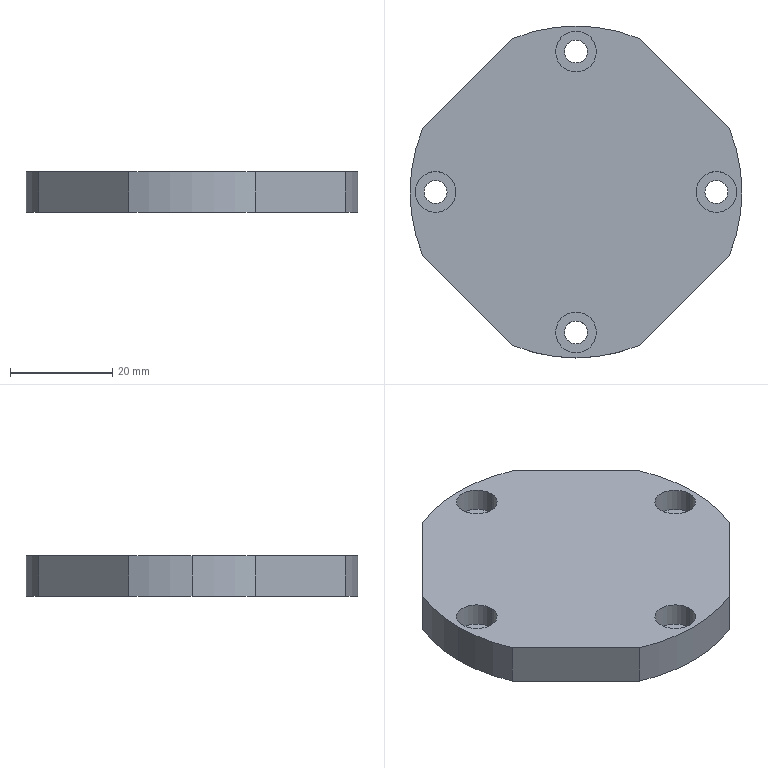Part | SolidWorks | features Extrusion 1, HoleWzd 1 | 1 solid | 31 faces | box 65 x 65 x 8 mm | volume 24061 mm3 | cylinder 21 | plane 10 | commonest cylinder face diameters 4.5 x8 8 x8 65 x5
STEP:
#1=CARTESIAN_POINT('',(-4.,27.5,3.4));
#2=VERTEX_POINT('',#1);
#3=CARTESIAN_POINT('',(4.,27.5,3.4));
#4=VERTEX_POINT('',#3);
#5=CARTESIAN_POINT('',(0.,27.5,3.4));
#6=DIRECTION('',(0.,0.,1.));
#7=DIRECTION('',(1.,0.,0.));
#8=AXIS2_PLACEMENT_3D('',#5,#6,#7);
#9=CIRCLE('',#8,4.);
#10=EDGE_CURVE('',#2,#4,#9,.T.);
#11=ORIENTED_EDGE('',*,*,#10,.F.);
#12=CARTESIAN_POINT('',(-4.,27.5,8.));
#13=VERTEX_POINT('',#12);
#14=CARTESIAN_POINT('',(-4.,27.5,8.));
#15=DIRECTION('',(0.,0.,1.));
#16=VECTOR('',#15,1000.);
#17=LINE('',#14,#16);
#18=EDGE_CURVE('',#2,#13,#17,.T.);
#19=ORIENTED_EDGE('',*,*,#18,.T.);
#20=CARTESIAN_POINT('',(4.,27.5,8.));
#21=VERTEX_POINT('',#20);
#22=CARTESIAN_POINT('',(0.,27.5,8.));
#23=DIRECTION('',(0.,0.,1.));
#24=DIRECTION('',(1.,0.,0.));
#25=AXIS2_PLACEMENT_3D('',#22,#23,#24);
#26=CIRCLE('',#25,4.);
#27=EDGE_CURVE('',#13,#21,#26,.T.);
#28=ORIENTED_EDGE('',*,*,#27,.T.);
#29=CARTESIAN_POINT('',(4.,27.5,8.));
#30=DIRECTION('',(0.,0.,1.));
#31=VECTOR('',#30,1000.);
#32=LINE('',#29,#31);
#33=EDGE_CURVE('',#4,#21,#32,.T.);
#34=ORIENTED_EDGE('',*,*,#33,.F.);
#35=EDGE_LOOP('',(#11,#19,#28,#34));
#36=FACE_OUTER_BOUND('',#35,.T.);
#37=CARTESIAN_POINT('',(0.,27.5,8.));
#38=DIRECTION('',(0.,0.,1.));
#39=DIRECTION('',(1.,0.,0.));
#40=AXIS2_PLACEMENT_3D('',#37,#38,#39);
#41=CYLINDRICAL_SURFACE('',#40,4.);
#42=ADVANCED_FACE('',(#36),#41,.F.);
#43=CARTESIAN_POINT('',(-2.25,27.5,0.));
#44=VERTEX_POINT('',#43);
#45=CARTESIAN_POINT('',(2.25,27.5,0.));
#46=VERTEX_POINT('',#45);
#47=CARTESIAN_POINT('',(0.,27.5,0.));
#48=DIRECTION('',(0.,0.,1.));
#49=DIRECTION('',(1.,0.,0.));
#50=AXIS2_PLACEMENT_3D('',#47,#48,#49);
#51=CIRCLE('',#50,2.25);
#52=EDGE_CURVE('',#44,#46,#51,.T.);
#53=ORIENTED_EDGE('',*,*,#52,.F.);
#54=CARTESIAN_POINT('',(-2.25,27.5,3.4));
#55=VERTEX_POINT('',#54);
#56=CARTESIAN_POINT('',(-2.25,27.5,8.));
#57=DIRECTION('',(0.,0.,1.));
#58=VECTOR('',#57,1000.);
#59=LINE('',#56,#58);
#60=EDGE_CURVE('',#44,#55,#59,.T.);
#61=ORIENTED_EDGE('',*,*,#60,.T.);
#62=CARTESIAN_POINT('',(2.25,27.5,3.4));
#63=VERTEX_POINT('',#62);
#64=CARTESIAN_POINT('',(0.,27.5,3.4));
#65=DIRECTION('',(0.,0.,1.));
#66=DIRECTION('',(1.,0.,0.));
#67=AXIS2_PLACEMENT_3D('',#64,#65,#66);
#68=CIRCLE('',#67,2.25);
#69=EDGE_CURVE('',#55,#63,#68,.T.);
#70=ORIENTED_EDGE('',*,*,#69,.T.);
#71=CARTESIAN_POINT('',(2.25,27.5,8.));
#72=DIRECTION('',(0.,0.,1.));
#73=VECTOR('',#72,1000.);
#74=LINE('',#71,#73);
#75=EDGE_CURVE('',#46,#63,#74,.T.);
#76=ORIENTED_EDGE('',*,*,#75,.F.);
#77=EDGE_LOOP('',(#53,#61,#70,#76));
#78=FACE_OUTER_BOUND('',#77,.T.);
#79=CARTESIAN_POINT('',(0.,27.5,8.));
#80=DIRECTION('',(0.,0.,1.));
#81=DIRECTION('',(1.,0.,0.));
#82=AXIS2_PLACEMENT_3D('',#79,#80,#81);
#83=CYLINDRICAL_SURFACE('',#82,2.25);
#84=ADVANCED_FACE('',(#78),#83,.F.);
#85=CARTESIAN_POINT('',(-31.5,0.,3.4));
#86=VERTEX_POINT('',#85);
#87=CARTESIAN_POINT('',(-23.5,0.,3.4));
#88=VERTEX_POINT('',#87);
#89=CARTESIAN_POINT('',(-27.5,0.,3.4));
#90=DIRECTION('',(0.,0.,1.));
#91=DIRECTION('',(1.,0.,0.));
#92=AXIS2_PLACEMENT_3D('',#89,#90,#91);
#93=CIRCLE('',#92,4.);
#94=EDGE_CURVE('',#86,#88,#93,.T.);
#95=ORIENTED_EDGE('',*,*,#94,.F.);
#96=CARTESIAN_POINT('',(-31.5,0.,8.));
#97=VERTEX_POINT('',#96);
#98=CARTESIAN_POINT('',(-31.5,0.,8.));
#99=DIRECTION('',(0.,0.,1.));
#100=VECTOR('',#99,1000.);
#101=LINE('',#98,#100);
#102=EDGE_CURVE('',#86,#97,#101,.T.);
#103=ORIENTED_EDGE('',*,*,#102,.T.);
#104=CARTESIAN_POINT('',(-23.5,0.,8.));
#105=VERTEX_POINT('',#104);
#106=CARTESIAN_POINT('',(-27.5,0.,8.));
#107=DIRECTION('',(0.,0.,1.));
#108=DIRECTION('',(1.,0.,0.));
#109=AXIS2_PLACEMENT_3D('',#106,#107,#108);
#110=CIRCLE('',#109,4.);
#111=EDGE_CURVE('',#97,#105,#110,.T.);
#112=ORIENTED_EDGE('',*,*,#111,.T.);
#113=CARTESIAN_POINT('',(-23.5,0.,8.));
#114=DIRECTION('',(0.,0.,1.));
#115=VECTOR('',#114,1000.);
#116=LINE('',#113,#115);
#117=EDGE_CURVE('',#88,#105,#116,.T.);
#118=ORIENTED_EDGE('',*,*,#117,.F.);
#119=EDGE_LOOP('',(#95,#103,#112,#118));
#120=FACE_OUTER_BOUND('',#119,.T.);
#121=CARTESIAN_POINT('',(-27.5,0.,8.));
#122=DIRECTION('',(0.,0.,1.));
#123=DIRECTION('',(1.,0.,0.));
#124=AXIS2_PLACEMENT_3D('',#121,#122,#123);
#125=CYLINDRICAL_SURFACE('',#124,4.);
#126=ADVANCED_FACE('',(#120),#125,.F.);
#127=CARTESIAN_POINT('',(-29.75,0.,0.));
#128=VERTEX_POINT('',#127);
#129=CARTESIAN_POINT('',(-25.25,0.,0.));
#130=VERTEX_POINT('',#129);
#131=CARTESIAN_POINT('',(-27.5,0.,0.));
#132=DIRECTION('',(0.,0.,1.));
#133=DIRECTION('',(1.,0.,0.));
#134=AXIS2_PLACEMENT_3D('',#131,#132,#133);
#135=CIRCLE('',#134,2.25);
#136=EDGE_CURVE('',#128,#130,#135,.T.);
#137=ORIENTED_EDGE('',*,*,#136,.F.);
#138=CARTESIAN_POINT('',(-29.75,0.,3.4));
#139=VERTEX_POINT('',#138);
#140=CARTESIAN_POINT('',(-29.75,0.,8.));
#141=DIRECTION('',(0.,0.,1.));
#142=VECTOR('',#141,1000.);
#143=LINE('',#140,#142);
#144=EDGE_CURVE('',#128,#139,#143,.T.);
#145=ORIENTED_EDGE('',*,*,#144,.T.);
#146=CARTESIAN_POINT('',(-25.25,0.,3.4));
#147=VERTEX_POINT('',#146);
#148=CARTESIAN_POINT('',(-27.5,0.,3.4));
#149=DIRECTION('',(0.,0.,1.));
#150=DIRECTION('',(1.,0.,0.));
#151=AXIS2_PLACEMENT_3D('',#148,#149,#150);
#152=CIRCLE('',#151,2.25);
#153=EDGE_CURVE('',#139,#147,#152,.T.);
#154=ORIENTED_EDGE('',*,*,#153,.T.);
#155=CARTESIAN_POINT('',(-25.25,0.,8.));
#156=DIRECTION('',(0.,0.,1.));
#157=VECTOR('',#156,1000.);
#158=LINE('',#155,#157);
#159=EDGE_CURVE('',#130,#147,#158,.T.);
#160=ORIENTED_EDGE('',*,*,#159,.F.);
#161=EDGE_LOOP('',(#137,#145,#154,#160));
#162=FACE_OUTER_BOUND('',#161,.T.);
#163=CARTESIAN_POINT('',(-27.5,0.,8.));
#164=DIRECTION('',(0.,0.,1.));
#165=DIRECTION('',(1.,0.,0.));
#166=AXIS2_PLACEMENT_3D('',#163,#164,#165);
#167=CYLINDRICAL_SURFACE('',#166,2.25);
#168=ADVANCED_FACE('',(#162),#167,.F.);
#169=CARTESIAN_POINT('',(-4.,-27.5,3.4));
#170=VERTEX_POINT('',#169);
#171=CARTESIAN_POINT('',(4.,-27.5,3.4));
#172=VERTEX_POINT('',#171);
#173=CARTESIAN_POINT('',(0.,-27.5,3.4));
#174=DIRECTION('',(0.,0.,1.));
#175=DIRECTION('',(1.,0.,0.));
#176=AXIS2_PLACEMENT_3D('',#173,#174,#175);
#177=CIRCLE('',#176,4.);
#178=EDGE_CURVE('',#170,#172,#177,.T.);
#179=ORIENTED_EDGE('',*,*,#178,.F.);
#180=CARTESIAN_POINT('',(-4.,-27.5,8.));
#181=VERTEX_POINT('',#180);
#182=CARTESIAN_POINT('',(-4.,-27.5,8.));
#183=DIRECTION('',(0.,0.,1.));
#184=VECTOR('',#183,1000.);
#185=LINE('',#182,#184);
#186=EDGE_CURVE('',#170,#181,#185,.T.);
#187=ORIENTED_EDGE('',*,*,#186,.T.);
#188=CARTESIAN_POINT('',(4.,-27.5,8.));
#189=VERTEX_POINT('',#188);
#190=CARTESIAN_POINT('',(0.,-27.5,8.));
#191=DIRECTION('',(0.,0.,1.));
#192=DIRECTION('',(1.,0.,0.));
#193=AXIS2_PLACEMENT_3D('',#190,#191,#192);
#194=CIRCLE('',#193,4.);
#195=EDGE_CURVE('',#181,#189,#194,.T.);
#196=ORIENTED_EDGE('',*,*,#195,.T.);
#197=CARTESIAN_POINT('',(4.,-27.5,8.));
#198=DIRECTION('',(0.,0.,1.));
#199=VECTOR('',#198,1000.);
#200=LINE('',#197,#199);
#201=EDGE_CURVE('',#172,#189,#200,.T.);
#202=ORIENTED_EDGE('',*,*,#201,.F.);
#203=EDGE_LOOP('',(#179,#187,#196,#202));
#204=FACE_OUTER_BOUND('',#203,.T.);
#205=CARTESIAN_POINT('',(0.,-27.5,8.));
#206=DIRECTION('',(0.,0.,1.));
#207=DIRECTION('',(1.,0.,0.));
#208=AXIS2_PLACEMENT_3D('',#205,#206,#207);
#209=CYLINDRICAL_SURFACE('',#208,4.);
#210=ADVANCED_FACE('',(#204),#209,.F.);
#211=CARTESIAN_POINT('',(-2.25,-27.5,0.));
#212=VERTEX_POINT('',#211);
#213=CARTESIAN_POINT('',(2.25,-27.5,0.));
#214=VERTEX_POINT('',#213);
#215=CARTESIAN_POINT('',(0.,-27.5,0.));
#216=DIRECTION('',(0.,0.,1.));
#217=DIRECTION('',(1.,0.,0.));
#218=AXIS2_PLACEMENT_3D('',#215,#216,#217);
#219=CIRCLE('',#218,2.25);
#220=EDGE_CURVE('',#212,#214,#219,.T.);
#221=ORIENTED_EDGE('',*,*,#220,.F.);
#222=CARTESIAN_POINT('',(-2.25,-27.5,3.4));
#223=VERTEX_POINT('',#222);
#224=CARTESIAN_POINT('',(-2.25,-27.5,8.));
#225=DIRECTION('',(0.,0.,1.));
#226=VECTOR('',#225,1000.);
#227=LINE('',#224,#226);
#228=EDGE_CURVE('',#212,#223,#227,.T.);
#229=ORIENTED_EDGE('',*,*,#228,.T.);
#230=CARTESIAN_POINT('',(2.25,-27.5,3.4));
#231=VERTEX_POINT('',#230);
#232=CARTESIAN_POINT('',(0.,-27.5,3.4));
#233=DIRECTION('',(0.,0.,1.));
#234=DIRECTION('',(1.,0.,0.));
#235=AXIS2_PLACEMENT_3D('',#232,#233,#234);
#236=CIRCLE('',#235,2.25);
#237=EDGE_CURVE('',#223,#231,#236,.T.);
#238=ORIENTED_EDGE('',*,*,#237,.T.);
#239=CARTESIAN_POINT('',(2.25,-27.5,8.));
#240=DIRECTION('',(0.,0.,1.));
#241=VECTOR('',#240,1000.);
#242=LINE('',#239,#241);
#243=EDGE_CURVE('',#214,#231,#242,.T.);
#244=ORIENTED_EDGE('',*,*,#243,.F.);
#245=EDGE_LOOP('',(#221,#229,#238,#244));
#246=FACE_OUTER_BOUND('',#245,.T.);
#247=CARTESIAN_POINT('',(0.,-27.5,8.));
#248=DIRECTION('',(0.,0.,1.));
#249=DIRECTION('',(1.,0.,0.));
#250=AXIS2_PLACEMENT_3D('',#247,#248,#249);
#251=CYLINDRICAL_SURFACE('',#250,2.25);
#252=ADVANCED_FACE('',(#246),#251,.F.);
#253=CARTESIAN_POINT('',(23.5,0.,3.4));
#254=VERTEX_POINT('',#253);
#255=CARTESIAN_POINT('',(31.5,0.,3.4));
#256=VERTEX_POINT('',#255);
#257=CARTESIAN_POINT('',(27.5,0.,3.4));
#258=DIRECTION('',(0.,0.,1.));
#259=DIRECTION('',(1.,0.,0.));
#260=AXIS2_PLACEMENT_3D('',#257,#258,#259);
#261=CIRCLE('',#260,4.);
#262=EDGE_CURVE('',#254,#256,#261,.T.);
#263=ORIENTED_EDGE('',*,*,#262,.F.);
#264=CARTESIAN_POINT('',(23.5,0.,8.));
#265=VERTEX_POINT('',#264);
#266=CARTESIAN_POINT('',(23.5,0.,8.));
#267=DIRECTION('',(0.,0.,1.));
#268=VECTOR('',#267,1000.);
#269=LINE('',#266,#268);
#270=EDGE_CURVE('',#254,#265,#269,.T.);
#271=ORIENTED_EDGE('',*,*,#270,.T.);
#272=CARTESIAN_POINT('',(31.5,0.,8.));
#273=VERTEX_POINT('',#272);
#274=CARTESIAN_POINT('',(27.5,0.,8.));
#275=DIRECTION('',(0.,0.,1.));
#276=DIRECTION('',(1.,0.,0.));
#277=AXIS2_PLACEMENT_3D('',#274,#275,#276);
#278=CIRCLE('',#277,4.);
#279=EDGE_CURVE('',#265,#273,#278,.T.);
#280=ORIENTED_EDGE('',*,*,#279,.T.);
#281=CARTESIAN_POINT('',(31.5,0.,8.));
#282=DIRECTION('',(0.,0.,1.));
#283=VECTOR('',#282,1000.);
#284=LINE('',#281,#283);
#285=EDGE_CURVE('',#256,#273,#284,.T.);
#286=ORIENTED_EDGE('',*,*,#285,.F.);
#287=EDGE_LOOP('',(#263,#271,#280,#286));
#288=FACE_OUTER_BOUND('',#287,.T.);
#289=CARTESIAN_POINT('',(27.5,0.,8.));
#290=DIRECTION('',(0.,0.,1.));
#291=DIRECTION('',(1.,0.,0.));
#292=AXIS2_PLACEMENT_3D('',#289,#290,#291);
#293=CYLINDRICAL_SURFACE('',#292,4.);
#294=ADVANCED_FACE('',(#288),#293,.F.);
#295=CARTESIAN_POINT('',(25.25,0.,0.));
#296=VERTEX_POINT('',#295);
#297=CARTESIAN_POINT('',(29.75,0.,0.));
#298=VERTEX_POINT('',#297);
#299=CARTESIAN_POINT('',(27.5,0.,0.));
#300=DIRECTION('',(0.,0.,1.));
#301=DIRECTION('',(1.,0.,0.));
#302=AXIS2_PLACEMENT_3D('',#299,#300,#301);
#303=CIRCLE('',#302,2.25);
#304=EDGE_CURVE('',#296,#298,#303,.T.);
#305=ORIENTED_EDGE('',*,*,#304,.F.);
#306=CARTESIAN_POINT('',(25.25,0.,3.4));
#307=VERTEX_POINT('',#306);
#308=CARTESIAN_POINT('',(25.25,0.,8.));
#309=DIRECTION('',(0.,0.,1.));
#310=VECTOR('',#309,1000.);
#311=LINE('',#308,#310);
#312=EDGE_CURVE('',#296,#307,#311,.T.);
#313=ORIENTED_EDGE('',*,*,#312,.T.);
#314=CARTESIAN_POINT('',(29.75,0.,3.4));
#315=VERTEX_POINT('',#314);
#316=CARTESIAN_POINT('',(27.5,0.,3.4));
#317=DIRECTION('',(0.,0.,1.));
#318=DIRECTION('',(1.,0.,0.));
#319=AXIS2_PLACEMENT_3D('',#316,#317,#318);
#320=CIRCLE('',#319,2.25);
#321=EDGE_CURVE('',#307,#315,#320,.T.);
#322=ORIENTED_EDGE('',*,*,#321,.T.);
#323=CARTESIAN_POINT('',(29.75,0.,8.));
#324=DIRECTION('',(0.,0.,1.));
#325=VECTOR('',#324,1000.);
#326=LINE('',#323,#325);
#327=EDGE_CURVE('',#298,#315,#326,.T.);
#328=ORIENTED_EDGE('',*,*,#327,.F.);
#329=EDGE_LOOP('',(#305,#313,#322,#328));
#330=FACE_OUTER_BOUND('',#329,.T.);
#331=CARTESIAN_POINT('',(27.5,0.,8.));
#332=DIRECTION('',(0.,0.,1.));
#333=DIRECTION('',(1.,0.,0.));
#334=AXIS2_PLACEMENT_3D('',#331,#332,#333);
#335=CYLINDRICAL_SURFACE('',#334,2.25);
#336=ADVANCED_FACE('',(#330),#335,.F.);
#337=CARTESIAN_POINT('',(-32.5,0.,8.));
#338=VERTEX_POINT('',#337);
#339=CARTESIAN_POINT('',(-30.052,-12.374,8.));
#340=VERTEX_POINT('',#339);
#341=CARTESIAN_POINT('',(0.,0.,8.));
#342=DIRECTION('',(0.,0.,1.));
#343=DIRECTION('',(1.,0.,0.));
#344=AXIS2_PLACEMENT_3D('',#341,#342,#343);
#345=CIRCLE('',#344,32.5);
#346=EDGE_CURVE('',#338,#340,#345,.T.);
#347=ORIENTED_EDGE('',*,*,#346,.F.);
#348=CARTESIAN_POINT('',(-32.5,0.,0.));
#349=VERTEX_POINT('',#348);
#350=CARTESIAN_POINT('',(-32.5,0.,8.));
#351=DIRECTION('',(0.,0.,-1.));
#352=VECTOR('',#351,1000.);
#353=LINE('',#350,#352);
#354=EDGE_CURVE('',#338,#349,#353,.T.);
#355=ORIENTED_EDGE('',*,*,#354,.T.);
#356=CARTESIAN_POINT('',(-30.052,-12.374,0.));
#357=VERTEX_POINT('',#356);
#358=CARTESIAN_POINT('',(0.,0.,0.));
#359=DIRECTION('',(0.,0.,1.));
#360=DIRECTION('',(1.,0.,0.));
#361=AXIS2_PLACEMENT_3D('',#358,#359,#360);
#362=CIRCLE('',#361,32.5);
#363=EDGE_CURVE('',#349,#357,#362,.T.);
#364=ORIENTED_EDGE('',*,*,#363,.T.);
#365=CARTESIAN_POINT('',(-30.052,-12.374,8.));
#366=DIRECTION('',(0.,0.,-1.));
#367=VECTOR('',#366,1000.);
#368=LINE('',#365,#367);
#369=EDGE_CURVE('',#340,#357,#368,.T.);
#370=ORIENTED_EDGE('',*,*,#369,.F.);
#371=EDGE_LOOP('',(#347,#355,#364,#370));
#372=FACE_OUTER_BOUND('',#371,.T.);
#373=CARTESIAN_POINT('',(0.,0.,8.));
#374=DIRECTION('',(0.,0.,-1.));
#375=DIRECTION('',(-1.,0.,0.));
#376=AXIS2_PLACEMENT_3D('',#373,#374,#375);
#377=CYLINDRICAL_SURFACE('',#376,32.5);
#378=ADVANCED_FACE('',(#372),#377,.T.);
#379=ORIENTED_EDGE('',*,*,#354,.F.);
#380=CARTESIAN_POINT('',(-30.052,12.374,8.));
#381=VERTEX_POINT('',#380);
#382=CARTESIAN_POINT('',(0.,0.,8.));
#383=DIRECTION('',(0.,0.,1.));
#384=DIRECTION('',(1.,0.,0.));
#385=AXIS2_PLACEMENT_3D('',#382,#383,#384);
#386=CIRCLE('',#385,32.5);
#387=EDGE_CURVE('',#381,#338,#386,.T.);
#388=ORIENTED_EDGE('',*,*,#387,.F.);
#389=CARTESIAN_POINT('',(-30.052,12.374,0.));
#390=VERTEX_POINT('',#389);
#391=CARTESIAN_POINT('',(-30.052,12.374,8.));
#392=DIRECTION('',(0.,0.,-1.));
#393=VECTOR('',#392,1000.);
#394=LINE('',#391,#393);
#395=EDGE_CURVE('',#381,#390,#394,.T.);
#396=ORIENTED_EDGE('',*,*,#395,.T.);
#397=CARTESIAN_POINT('',(0.,0.,0.));
#398=DIRECTION('',(0.,0.,1.));
#399=DIRECTION('',(1.,0.,0.));
#400=AXIS2_PLACEMENT_3D('',#397,#398,#399);
#401=CIRCLE('',#400,32.5);
#402=EDGE_CURVE('',#390,#349,#401,.T.);
#403=ORIENTED_EDGE('',*,*,#402,.T.);
#404=EDGE_LOOP('',(#379,#388,#396,#403));
#405=FACE_OUTER_BOUND('',#404,.T.);
#406=CARTESIAN_POINT('',(0.,0.,8.));
#407=DIRECTION('',(0.,0.,-1.));
#408=DIRECTION('',(-1.,0.,0.));
#409=AXIS2_PLACEMENT_3D('',#406,#407,#408);
#410=CYLINDRICAL_SURFACE('',#409,32.5);
#411=ADVANCED_FACE('',(#405),#410,.T.);
#412=CARTESIAN_POINT('',(-12.374,-30.052,0.));
#413=VERTEX_POINT('',#412);
#414=CARTESIAN_POINT('',(-30.052,-12.374,0.));
#415=DIRECTION('',(0.7071,-0.7071,0.));
#416=VECTOR('',#415,1000.);
#417=LINE('',#414,#416);
#418=EDGE_CURVE('',#357,#413,#417,.T.);
#419=ORIENTED_EDGE('',*,*,#418,.T.);
#420=CARTESIAN_POINT('',(-12.374,-30.052,8.));
#421=VERTEX_POINT('',#420);
#422=CARTESIAN_POINT('',(-12.374,-30.052,8.));
#423=DIRECTION('',(0.,0.,-1.));
#424=VECTOR('',#423,1000.);
#425=LINE('',#422,#424);
#426=EDGE_CURVE('',#421,#413,#425,.T.);
#427=ORIENTED_EDGE('',*,*,#426,.F.);
#428=CARTESIAN_POINT('',(-30.052,-12.374,8.));
#429=DIRECTION('',(0.7071,-0.7071,0.));
#430=VECTOR('',#429,1000.);
#431=LINE('',#428,#430);
#432=EDGE_CURVE('',#340,#421,#431,.T.);
#433=ORIENTED_EDGE('',*,*,#432,.F.);
#434=ORIENTED_EDGE('',*,*,#369,.T.);
#435=EDGE_LOOP('',(#419,#427,#433,#434));
#436=FACE_OUTER_BOUND('',#435,.T.);
#437=CARTESIAN_POINT('',(-30.052,-12.374,8.));
#438=DIRECTION('',(0.7071,0.7071,0.));
#439=DIRECTION('',(-0.7071,0.7071,0.));
#440=AXIS2_PLACEMENT_3D('',#437,#438,#439);
#441=PLANE('',#440);
#442=ADVANCED_FACE('',(#436),#441,.F.);
#443=CARTESIAN_POINT('',(12.374,-30.052,0.));
#444=VERTEX_POINT('',#443);
#445=CARTESIAN_POINT('',(0.,0.,0.));
#446=DIRECTION('',(0.,0.,1.));
#447=DIRECTION('',(1.,0.,0.));
#448=AXIS2_PLACEMENT_3D('',#445,#446,#447);
#449=CIRCLE('',#448,32.5);
#450=EDGE_CURVE('',#413,#444,#449,.T.);
#451=ORIENTED_EDGE('',*,*,#450,.T.);
#452=CARTESIAN_POINT('',(12.374,-30.052,8.));
#453=VERTEX_POINT('',#452);
#454=CARTESIAN_POINT('',(12.374,-30.052,8.));
#455=DIRECTION('',(0.,0.,-1.));
#456=VECTOR('',#455,1000.);
#457=LINE('',#454,#456);
#458=EDGE_CURVE('',#453,#444,#457,.T.);
#459=ORIENTED_EDGE('',*,*,#458,.F.);
#460=CARTESIAN_POINT('',(0.,0.,8.));
#461=DIRECTION('',(0.,0.,1.));
#462=DIRECTION('',(1.,0.,0.));
#463=AXIS2_PLACEMENT_3D('',#460,#461,#462);
#464=CIRCLE('',#463,32.5);
#465=EDGE_CURVE('',#421,#453,#464,.T.);
#466=ORIENTED_EDGE('',*,*,#465,.F.);
#467=ORIENTED_EDGE('',*,*,#426,.T.);
#468=EDGE_LOOP('',(#451,#459,#466,#467));
#469=FACE_OUTER_BOUND('',#468,.T.);
#470=CARTESIAN_POINT('',(0.,0.,8.));
#471=DIRECTION('',(0.,0.,-1.));
#472=DIRECTION('',(-1.,0.,0.));
#473=AXIS2_PLACEMENT_3D('',#470,#471,#472);
#474=CYLINDRICAL_SURFACE('',#473,32.5);
#475=ADVANCED_FACE('',(#469),#474,.T.);
#476=CARTESIAN_POINT('',(30.052,-12.374,0.));
#477=VERTEX_POINT('',#476);
#478=CARTESIAN_POINT('',(12.374,-30.052,0.));
#479=DIRECTION('',(0.7071,0.7071,0.));
#480=VECTOR('',#479,1000.);
#481=LINE('',#478,#480);
#482=EDGE_CURVE('',#444,#477,#481,.T.);
#483=ORIENTED_EDGE('',*,*,#482,.T.);
#484=CARTESIAN_POINT('',(30.052,-12.374,8.));
#485=VERTEX_POINT('',#484);
#486=CARTESIAN_POINT('',(30.052,-12.374,8.));
#487=DIRECTION('',(0.,0.,-1.));
#488=VECTOR('',#487,1000.);
#489=LINE('',#486,#488);
#490=EDGE_CURVE('',#485,#477,#489,.T.);
#491=ORIENTED_EDGE('',*,*,#490,.F.);
#492=CARTESIAN_POINT('',(12.374,-30.052,8.));
#493=DIRECTION('',(0.7071,0.7071,0.));
#494=VECTOR('',#493,1000.);
#495=LINE('',#492,#494);
#496=EDGE_CURVE('',#453,#485,#495,.T.);
#497=ORIENTED_EDGE('',*,*,#496,.F.);
#498=ORIENTED_EDGE('',*,*,#458,.T.);
#499=EDGE_LOOP('',(#483,#491,#497,#498));
#500=FACE_OUTER_BOUND('',#499,.T.);
#501=CARTESIAN_POINT('',(12.374,-30.052,8.));
#502=DIRECTION('',(-0.7071,0.7071,0.));
#503=DIRECTION('',(-0.7071,-0.7071,0.));
#504=AXIS2_PLACEMENT_3D('',#501,#502,#503);
#505=PLANE('',#504);
#506=ADVANCED_FACE('',(#500),#505,.F.);
#507=CARTESIAN_POINT('',(30.052,12.374,0.));
#508=VERTEX_POINT('',#507);
#509=CARTESIAN_POINT('',(0.,0.,0.));
#510=DIRECTION('',(0.,0.,1.));
#511=DIRECTION('',(1.,0.,0.));
#512=AXIS2_PLACEMENT_3D('',#509,#510,#511);
#513=CIRCLE('',#512,32.5);
#514=EDGE_CURVE('',#477,#508,#513,.T.);
#515=ORIENTED_EDGE('',*,*,#514,.T.);
#516=CARTESIAN_POINT('',(30.052,12.374,8.));
#517=VERTEX_POINT('',#516);
#518=CARTESIAN_POINT('',(30.052,12.374,8.));
#519=DIRECTION('',(0.,0.,-1.));
#520=VECTOR('',#519,1000.);
#521=LINE('',#518,#520);
#522=EDGE_CURVE('',#517,#508,#521,.T.);
#523=ORIENTED_EDGE('',*,*,#522,.F.);
#524=CARTESIAN_POINT('',(0.,0.,8.));
#525=DIRECTION('',(0.,0.,1.));
#526=DIRECTION('',(1.,0.,0.));
#527=AXIS2_PLACEMENT_3D('',#524,#525,#526);
#528=CIRCLE('',#527,32.5);
#529=EDGE_CURVE('',#485,#517,#528,.T.);
#530=ORIENTED_EDGE('',*,*,#529,.F.);
#531=ORIENTED_EDGE('',*,*,#490,.T.);
#532=EDGE_LOOP('',(#515,#523,#530,#531));
#533=FACE_OUTER_BOUND('',#532,.T.);
#534=CARTESIAN_POINT('',(0.,0.,8.));
#535=DIRECTION('',(0.,0.,-1.));
#536=DIRECTION('',(-1.,0.,0.));
#537=AXIS2_PLACEMENT_3D('',#534,#535,#536);
#538=CYLINDRICAL_SURFACE('',#537,32.5);
#539=ADVANCED_FACE('',(#533),#538,.T.);
#540=CARTESIAN_POINT('',(12.374,30.052,0.));
#541=VERTEX_POINT('',#540);
#542=CARTESIAN_POINT('',(12.374,30.052,0.));
#543=DIRECTION('',(-0.7071,0.7071,0.));
#544=VECTOR('',#543,1000.);
#545=LINE('',#542,#544);
#546=EDGE_CURVE('',#508,#541,#545,.T.);
#547=ORIENTED_EDGE('',*,*,#546,.T.);
#548=CARTESIAN_POINT('',(12.374,30.052,8.));
#549=VERTEX_POINT('',#548);
#550=CARTESIAN_POINT('',(12.374,30.052,8.));
#551=DIRECTION('',(0.,0.,-1.));
#552=VECTOR('',#551,1000.);
#553=LINE('',#550,#552);
#554=EDGE_CURVE('',#549,#541,#553,.T.);
#555=ORIENTED_EDGE('',*,*,#554,.F.);
#556=CARTESIAN_POINT('',(12.374,30.052,8.));
#557=DIRECTION('',(-0.7071,0.7071,0.));
#558=VECTOR('',#557,1000.);
#559=LINE('',#556,#558);
#560=EDGE_CURVE('',#517,#549,#559,.T.);
#561=ORIENTED_EDGE('',*,*,#560,.F.);
#562=ORIENTED_EDGE('',*,*,#522,.T.);
#563=EDGE_LOOP('',(#547,#555,#561,#562));
#564=FACE_OUTER_BOUND('',#563,.T.);
#565=CARTESIAN_POINT('',(12.374,30.052,8.));
#566=DIRECTION('',(-0.7071,-0.7071,0.));
#567=DIRECTION('',(0.7071,-0.7071,0.));
#568=AXIS2_PLACEMENT_3D('',#565,#566,#567);
#569=PLANE('',#568);
#570=ADVANCED_FACE('',(#564),#569,.F.);
#571=CARTESIAN_POINT('',(-12.374,30.052,0.));
#572=VERTEX_POINT('',#571);
#573=CARTESIAN_POINT('',(0.,0.,0.));
#574=DIRECTION('',(0.,0.,1.));
#575=DIRECTION('',(1.,0.,0.));
#576=AXIS2_PLACEMENT_3D('',#573,#574,#575);
#577=CIRCLE('',#576,32.5);
#578=EDGE_CURVE('',#541,#572,#577,.T.);
#579=ORIENTED_EDGE('',*,*,#578,.T.);
#580=CARTESIAN_POINT('',(-12.374,30.052,8.));
#581=VERTEX_POINT('',#580);
#582=CARTESIAN_POINT('',(-12.374,30.052,8.));
#583=DIRECTION('',(0.,0.,-1.));
#584=VECTOR('',#583,1000.);
#585=LINE('',#582,#584);
#586=EDGE_CURVE('',#581,#572,#585,.T.);
#587=ORIENTED_EDGE('',*,*,#586,.F.);
#588=CARTESIAN_POINT('',(0.,0.,8.));
#589=DIRECTION('',(0.,0.,1.));
#590=DIRECTION('',(1.,0.,0.));
#591=AXIS2_PLACEMENT_3D('',#588,#589,#590);
#592=CIRCLE('',#591,32.5);
#593=EDGE_CURVE('',#549,#581,#592,.T.);
#594=ORIENTED_EDGE('',*,*,#593,.F.);
#595=ORIENTED_EDGE('',*,*,#554,.T.);
#596=EDGE_LOOP('',(#579,#587,#594,#595));
#597=FACE_OUTER_BOUND('',#596,.T.);
#598=CARTESIAN_POINT('',(0.,0.,8.));
#599=DIRECTION('',(0.,0.,-1.));
#600=DIRECTION('',(-1.,0.,0.));
#601=AXIS2_PLACEMENT_3D('',#598,#599,#600);
#602=CYLINDRICAL_SURFACE('',#601,32.5);
#603=ADVANCED_FACE('',(#597),#602,.T.);
#604=CARTESIAN_POINT('',(-30.052,12.374,0.));
#605=DIRECTION('',(-0.7071,-0.7071,0.));
#606=VECTOR('',#605,1000.);
#607=LINE('',#604,#606);
#608=EDGE_CURVE('',#572,#390,#607,.T.);
#609=ORIENTED_EDGE('',*,*,#608,.T.);
#610=ORIENTED_EDGE('',*,*,#395,.F.);
#611=CARTESIAN_POINT('',(-30.052,12.374,8.));
#612=DIRECTION('',(-0.7071,-0.7071,0.));
#613=VECTOR('',#612,1000.);
#614=LINE('',#611,#613);
#615=EDGE_CURVE('',#581,#381,#614,.T.);
#616=ORIENTED_EDGE('',*,*,#615,.F.);
#617=ORIENTED_EDGE('',*,*,#586,.T.);
#618=EDGE_LOOP('',(#609,#610,#616,#617));
#619=FACE_OUTER_BOUND('',#618,.T.);
#620=CARTESIAN_POINT('',(-30.052,12.374,8.));
#621=DIRECTION('',(0.7071,-0.7071,0.));
#622=DIRECTION('',(0.7071,0.7071,0.));
#623=AXIS2_PLACEMENT_3D('',#620,#621,#622);
#624=PLANE('',#623);
#625=ADVANCED_FACE('',(#619),#624,.F.);
#626=CARTESIAN_POINT('',(0.,27.5,8.));
#627=DIRECTION('',(0.,0.,1.));
#628=DIRECTION('',(1.,0.,0.));
#629=AXIS2_PLACEMENT_3D('',#626,#627,#628);
#630=CIRCLE('',#629,4.);
#631=EDGE_CURVE('',#21,#13,#630,.T.);
#632=ORIENTED_EDGE('',*,*,#631,.F.);
#633=ORIENTED_EDGE('',*,*,#27,.F.);
#634=EDGE_LOOP('',(#632,#633));
#635=FACE_BOUND('',#634,.T.);
#636=CARTESIAN_POINT('',(-27.5,0.,8.));
#637=DIRECTION('',(0.,0.,1.));
#638=DIRECTION('',(1.,0.,0.));
#639=AXIS2_PLACEMENT_3D('',#636,#637,#638);
#640=CIRCLE('',#639,4.);
#641=EDGE_CURVE('',#105,#97,#640,.T.);
#642=ORIENTED_EDGE('',*,*,#641,.F.);
#643=ORIENTED_EDGE('',*,*,#111,.F.);
#644=EDGE_LOOP('',(#642,#643));
#645=FACE_BOUND('',#644,.T.);
#646=CARTESIAN_POINT('',(0.,-27.5,8.));
#647=DIRECTION('',(0.,0.,1.));
#648=DIRECTION('',(1.,0.,0.));
#649=AXIS2_PLACEMENT_3D('',#646,#647,#648);
#650=CIRCLE('',#649,4.);
#651=EDGE_CURVE('',#189,#181,#650,.T.);
#652=ORIENTED_EDGE('',*,*,#651,.F.);
#653=ORIENTED_EDGE('',*,*,#195,.F.);
#654=EDGE_LOOP('',(#652,#653));
#655=FACE_BOUND('',#654,.T.);
#656=CARTESIAN_POINT('',(27.5,0.,8.));
#657=DIRECTION('',(0.,0.,1.));
#658=DIRECTION('',(1.,0.,0.));
#659=AXIS2_PLACEMENT_3D('',#656,#657,#658);
#660=CIRCLE('',#659,4.);
#661=EDGE_CURVE('',#273,#265,#660,.T.);
#662=ORIENTED_EDGE('',*,*,#661,.F.);
#663=ORIENTED_EDGE('',*,*,#279,.F.);
#664=EDGE_LOOP('',(#662,#663));
#665=FACE_BOUND('',#664,.T.);
#666=ORIENTED_EDGE('',*,*,#387,.T.);
#667=ORIENTED_EDGE('',*,*,#346,.T.);
#668=ORIENTED_EDGE('',*,*,#432,.T.);
#669=ORIENTED_EDGE('',*,*,#465,.T.);
#670=ORIENTED_EDGE('',*,*,#496,.T.);
#671=ORIENTED_EDGE('',*,*,#529,.T.);
#672=ORIENTED_EDGE('',*,*,#560,.T.);
#673=ORIENTED_EDGE('',*,*,#593,.T.);
#674=ORIENTED_EDGE('',*,*,#615,.T.);
#675=EDGE_LOOP('',(#666,#667,#668,#669,#670,#671,#672,#673,#674));
#676=FACE_OUTER_BOUND('',#675,.T.);
#677=CARTESIAN_POINT('',(0.,0.,8.));
#678=DIRECTION('',(0.,0.,1.));
#679=DIRECTION('',(1.,0.,0.));
#680=AXIS2_PLACEMENT_3D('',#677,#678,#679);
#681=PLANE('',#680);
#682=ADVANCED_FACE('',(#635,#645,#655,#665,#676),#681,.T.);
#683=CARTESIAN_POINT('',(0.,27.5,0.));
#684=DIRECTION('',(0.,0.,1.));
#685=DIRECTION('',(1.,0.,0.));
#686=AXIS2_PLACEMENT_3D('',#683,#684,#685);
#687=CIRCLE('',#686,2.25);
#688=EDGE_CURVE('',#46,#44,#687,.T.);
#689=ORIENTED_EDGE('',*,*,#688,.T.);
#690=ORIENTED_EDGE('',*,*,#52,.T.);
#691=EDGE_LOOP('',(#689,#690));
#692=FACE_BOUND('',#691,.T.);
#693=CARTESIAN_POINT('',(-27.5,0.,0.));
#694=DIRECTION('',(0.,0.,1.));
#695=DIRECTION('',(1.,0.,0.));
#696=AXIS2_PLACEMENT_3D('',#693,#694,#695);
#697=CIRCLE('',#696,2.25);
#698=EDGE_CURVE('',#130,#128,#697,.T.);
#699=ORIENTED_EDGE('',*,*,#698,.T.);
#700=ORIENTED_EDGE('',*,*,#136,.T.);
#701=EDGE_LOOP('',(#699,#700));
#702=FACE_BOUND('',#701,.T.);
#703=CARTESIAN_POINT('',(0.,-27.5,0.));
#704=DIRECTION('',(0.,0.,1.));
#705=DIRECTION('',(1.,0.,0.));
#706=AXIS2_PLACEMENT_3D('',#703,#704,#705);
#707=CIRCLE('',#706,2.25);
#708=EDGE_CURVE('',#214,#212,#707,.T.);
#709=ORIENTED_EDGE('',*,*,#708,.T.);
#710=ORIENTED_EDGE('',*,*,#220,.T.);
#711=EDGE_LOOP('',(#709,#710));
#712=FACE_BOUND('',#711,.T.);
#713=CARTESIAN_POINT('',(27.5,0.,0.));
#714=DIRECTION('',(0.,0.,1.));
#715=DIRECTION('',(1.,0.,0.));
#716=AXIS2_PLACEMENT_3D('',#713,#714,#715);
#717=CIRCLE('',#716,2.25);
#718=EDGE_CURVE('',#298,#296,#717,.T.);
#719=ORIENTED_EDGE('',*,*,#718,.T.);
#720=ORIENTED_EDGE('',*,*,#304,.T.);
#721=EDGE_LOOP('',(#719,#720));
#722=FACE_BOUND('',#721,.T.);
#723=ORIENTED_EDGE('',*,*,#402,.F.);
#724=ORIENTED_EDGE('',*,*,#608,.F.);
#725=ORIENTED_EDGE('',*,*,#578,.F.);
#726=ORIENTED_EDGE('',*,*,#546,.F.);
#727=ORIENTED_EDGE('',*,*,#514,.F.);
#728=ORIENTED_EDGE('',*,*,#482,.F.);
#729=ORIENTED_EDGE('',*,*,#450,.F.);
#730=ORIENTED_EDGE('',*,*,#418,.F.);
#731=ORIENTED_EDGE('',*,*,#363,.F.);
#732=EDGE_LOOP('',(#723,#724,#725,#726,#727,#728,#729,#730,#731));
#733=FACE_OUTER_BOUND('',#732,.T.);
#734=CARTESIAN_POINT('',(0.,0.,0.));
#735=DIRECTION('',(0.,0.,1.));
#736=DIRECTION('',(1.,0.,0.));
#737=AXIS2_PLACEMENT_3D('',#734,#735,#736);
#738=PLANE('',#737);
#739=ADVANCED_FACE('',(#692,#702,#712,#722,#733),#738,.F.);
#740=ORIENTED_EDGE('',*,*,#312,.F.);
#741=ORIENTED_EDGE('',*,*,#718,.F.);
#742=ORIENTED_EDGE('',*,*,#327,.T.);
#743=CARTESIAN_POINT('',(27.5,0.,3.4));
#744=DIRECTION('',(0.,0.,1.));
#745=DIRECTION('',(1.,0.,0.));
#746=AXIS2_PLACEMENT_3D('',#743,#744,#745);
#747=CIRCLE('',#746,2.25);
#748=EDGE_CURVE('',#315,#307,#747,.T.);
#749=ORIENTED_EDGE('',*,*,#748,.T.);
#750=EDGE_LOOP('',(#740,#741,#742,#749));
#751=FACE_OUTER_BOUND('',#750,.T.);
#752=CARTESIAN_POINT('',(27.5,0.,8.));
#753=DIRECTION('',(0.,0.,1.));
#754=DIRECTION('',(1.,0.,0.));
#755=AXIS2_PLACEMENT_3D('',#752,#753,#754);
#756=CYLINDRICAL_SURFACE('',#755,2.25);
#757=ADVANCED_FACE('',(#751),#756,.F.);
#758=ORIENTED_EDGE('',*,*,#748,.F.);
#759=ORIENTED_EDGE('',*,*,#321,.F.);
#760=EDGE_LOOP('',(#758,#759));
#761=FACE_BOUND('',#760,.T.);
#762=CARTESIAN_POINT('',(27.5,0.,3.4));
#763=DIRECTION('',(0.,0.,1.));
#764=DIRECTION('',(1.,0.,0.));
#765=AXIS2_PLACEMENT_3D('',#762,#763,#764);
#766=CIRCLE('',#765,4.);
#767=EDGE_CURVE('',#256,#254,#766,.T.);
#768=ORIENTED_EDGE('',*,*,#767,.T.);
#769=ORIENTED_EDGE('',*,*,#262,.T.);
#770=EDGE_LOOP('',(#768,#769));
#771=FACE_OUTER_BOUND('',#770,.T.);
#772=CARTESIAN_POINT('',(29.75,0.,3.4));
#773=DIRECTION('',(0.,0.,-1.));
#774=DIRECTION('',(-1.,0.,0.));
#775=AXIS2_PLACEMENT_3D('',#772,#773,#774);
#776=PLANE('',#775);
#777=ADVANCED_FACE('',(#761,#771),#776,.F.);
#778=ORIENTED_EDGE('',*,*,#270,.F.);
#779=ORIENTED_EDGE('',*,*,#767,.F.);
#780=ORIENTED_EDGE('',*,*,#285,.T.);
#781=ORIENTED_EDGE('',*,*,#661,.T.);
#782=EDGE_LOOP('',(#778,#779,#780,#781));
#783=FACE_OUTER_BOUND('',#782,.T.);
#784=CARTESIAN_POINT('',(27.5,0.,8.));
#785=DIRECTION('',(0.,0.,1.));
#786=DIRECTION('',(1.,0.,0.));
#787=AXIS2_PLACEMENT_3D('',#784,#785,#786);
#788=CYLINDRICAL_SURFACE('',#787,4.);
#789=ADVANCED_FACE('',(#783),#788,.F.);
#790=ORIENTED_EDGE('',*,*,#228,.F.);
#791=ORIENTED_EDGE('',*,*,#708,.F.);
#792=ORIENTED_EDGE('',*,*,#243,.T.);
#793=CARTESIAN_POINT('',(0.,-27.5,3.4));
#794=DIRECTION('',(0.,0.,1.));
#795=DIRECTION('',(1.,0.,0.));
#796=AXIS2_PLACEMENT_3D('',#793,#794,#795);
#797=CIRCLE('',#796,2.25);
#798=EDGE_CURVE('',#231,#223,#797,.T.);
#799=ORIENTED_EDGE('',*,*,#798,.T.);
#800=EDGE_LOOP('',(#790,#791,#792,#799));
#801=FACE_OUTER_BOUND('',#800,.T.);
#802=CARTESIAN_POINT('',(0.,-27.5,8.));
#803=DIRECTION('',(0.,0.,1.));
#804=DIRECTION('',(1.,0.,0.));
#805=AXIS2_PLACEMENT_3D('',#802,#803,#804);
#806=CYLINDRICAL_SURFACE('',#805,2.25);
#807=ADVANCED_FACE('',(#801),#806,.F.);
#808=ORIENTED_EDGE('',*,*,#798,.F.);
#809=ORIENTED_EDGE('',*,*,#237,.F.);
#810=EDGE_LOOP('',(#808,#809));
#811=FACE_BOUND('',#810,.T.);
#812=CARTESIAN_POINT('',(0.,-27.5,3.4));
#813=DIRECTION('',(0.,0.,1.));
#814=DIRECTION('',(1.,0.,0.));
#815=AXIS2_PLACEMENT_3D('',#812,#813,#814);
#816=CIRCLE('',#815,4.);
#817=EDGE_CURVE('',#172,#170,#816,.T.);
#818=ORIENTED_EDGE('',*,*,#817,.T.);
#819=ORIENTED_EDGE('',*,*,#178,.T.);
#820=EDGE_LOOP('',(#818,#819));
#821=FACE_OUTER_BOUND('',#820,.T.);
#822=CARTESIAN_POINT('',(2.25,-27.5,3.4));
#823=DIRECTION('',(0.,0.,-1.));
#824=DIRECTION('',(-1.,0.,0.));
#825=AXIS2_PLACEMENT_3D('',#822,#823,#824);
#826=PLANE('',#825);
#827=ADVANCED_FACE('',(#811,#821),#826,.F.);
#828=ORIENTED_EDGE('',*,*,#186,.F.);
#829=ORIENTED_EDGE('',*,*,#817,.F.);
#830=ORIENTED_EDGE('',*,*,#201,.T.);
#831=ORIENTED_EDGE('',*,*,#651,.T.);
#832=EDGE_LOOP('',(#828,#829,#830,#831));
#833=FACE_OUTER_BOUND('',#832,.T.);
#834=CARTESIAN_POINT('',(0.,-27.5,8.));
#835=DIRECTION('',(0.,0.,1.));
#836=DIRECTION('',(1.,0.,0.));
#837=AXIS2_PLACEMENT_3D('',#834,#835,#836);
#838=CYLINDRICAL_SURFACE('',#837,4.);
#839=ADVANCED_FACE('',(#833),#838,.F.);
#840=ORIENTED_EDGE('',*,*,#144,.F.);
#841=ORIENTED_EDGE('',*,*,#698,.F.);
#842=ORIENTED_EDGE('',*,*,#159,.T.);
#843=CARTESIAN_POINT('',(-27.5,0.,3.4));
#844=DIRECTION('',(0.,0.,1.));
#845=DIRECTION('',(1.,0.,0.));
#846=AXIS2_PLACEMENT_3D('',#843,#844,#845);
#847=CIRCLE('',#846,2.25);
#848=EDGE_CURVE('',#147,#139,#847,.T.);
#849=ORIENTED_EDGE('',*,*,#848,.T.);
#850=EDGE_LOOP('',(#840,#841,#842,#849));
#851=FACE_OUTER_BOUND('',#850,.T.);
#852=CARTESIAN_POINT('',(-27.5,0.,8.));
#853=DIRECTION('',(0.,0.,1.));
#854=DIRECTION('',(1.,0.,0.));
#855=AXIS2_PLACEMENT_3D('',#852,#853,#854);
#856=CYLINDRICAL_SURFACE('',#855,2.25);
#857=ADVANCED_FACE('',(#851),#856,.F.);
#858=ORIENTED_EDGE('',*,*,#848,.F.);
#859=ORIENTED_EDGE('',*,*,#153,.F.);
#860=EDGE_LOOP('',(#858,#859));
#861=FACE_BOUND('',#860,.T.);
#862=CARTESIAN_POINT('',(-27.5,0.,3.4));
#863=DIRECTION('',(0.,0.,1.));
#864=DIRECTION('',(1.,0.,0.));
#865=AXIS2_PLACEMENT_3D('',#862,#863,#864);
#866=CIRCLE('',#865,4.);
#867=EDGE_CURVE('',#88,#86,#866,.T.);
#868=ORIENTED_EDGE('',*,*,#867,.T.);
#869=ORIENTED_EDGE('',*,*,#94,.T.);
#870=EDGE_LOOP('',(#868,#869));
#871=FACE_OUTER_BOUND('',#870,.T.);
#872=CARTESIAN_POINT('',(-25.25,0.,3.4));
#873=DIRECTION('',(0.,0.,-1.));
#874=DIRECTION('',(-1.,0.,0.));
#875=AXIS2_PLACEMENT_3D('',#872,#873,#874);
#876=PLANE('',#875);
#877=ADVANCED_FACE('',(#861,#871),#876,.F.);
#878=ORIENTED_EDGE('',*,*,#102,.F.);
#879=ORIENTED_EDGE('',*,*,#867,.F.);
#880=ORIENTED_EDGE('',*,*,#117,.T.);
#881=ORIENTED_EDGE('',*,*,#641,.T.);
#882=EDGE_LOOP('',(#878,#879,#880,#881));
#883=FACE_OUTER_BOUND('',#882,.T.);
#884=CARTESIAN_POINT('',(-27.5,0.,8.));
#885=DIRECTION('',(0.,0.,1.));
#886=DIRECTION('',(1.,0.,0.));
#887=AXIS2_PLACEMENT_3D('',#884,#885,#886);
#888=CYLINDRICAL_SURFACE('',#887,4.);
#889=ADVANCED_FACE('',(#883),#888,.F.);
#890=ORIENTED_EDGE('',*,*,#60,.F.);
#891=ORIENTED_EDGE('',*,*,#688,.F.);
#892=ORIENTED_EDGE('',*,*,#75,.T.);
#893=CARTESIAN_POINT('',(0.,27.5,3.4));
#894=DIRECTION('',(0.,0.,1.));
#895=DIRECTION('',(1.,0.,0.));
#896=AXIS2_PLACEMENT_3D('',#893,#894,#895);
#897=CIRCLE('',#896,2.25);
#898=EDGE_CURVE('',#63,#55,#897,.T.);
#899=ORIENTED_EDGE('',*,*,#898,.T.);
#900=EDGE_LOOP('',(#890,#891,#892,#899));
#901=FACE_OUTER_BOUND('',#900,.T.);
#902=CARTESIAN_POINT('',(0.,27.5,8.));
#903=DIRECTION('',(0.,0.,1.));
#904=DIRECTION('',(1.,0.,0.));
#905=AXIS2_PLACEMENT_3D('',#902,#903,#904);
#906=CYLINDRICAL_SURFACE('',#905,2.25);
#907=ADVANCED_FACE('',(#901),#906,.F.);
#908=ORIENTED_EDGE('',*,*,#898,.F.);
#909=ORIENTED_EDGE('',*,*,#69,.F.);
#910=EDGE_LOOP('',(#908,#909));
#911=FACE_BOUND('',#910,.T.);
#912=CARTESIAN_POINT('',(0.,27.5,3.4));
#913=DIRECTION('',(0.,0.,1.));
#914=DIRECTION('',(1.,0.,0.));
#915=AXIS2_PLACEMENT_3D('',#912,#913,#914);
#916=CIRCLE('',#915,4.);
#917=EDGE_CURVE('',#4,#2,#916,.T.);
#918=ORIENTED_EDGE('',*,*,#917,.T.);
#919=ORIENTED_EDGE('',*,*,#10,.T.);
#920=EDGE_LOOP('',(#918,#919));
#921=FACE_OUTER_BOUND('',#920,.T.);
#922=CARTESIAN_POINT('',(2.25,27.5,3.4));
#923=DIRECTION('',(0.,0.,-1.));
#924=DIRECTION('',(-1.,0.,0.));
#925=AXIS2_PLACEMENT_3D('',#922,#923,#924);
#926=PLANE('',#925);
#927=ADVANCED_FACE('',(#911,#921),#926,.F.);
#928=ORIENTED_EDGE('',*,*,#18,.F.);
#929=ORIENTED_EDGE('',*,*,#917,.F.);
#930=ORIENTED_EDGE('',*,*,#33,.T.);
#931=ORIENTED_EDGE('',*,*,#631,.T.);
#932=EDGE_LOOP('',(#928,#929,#930,#931));
#933=FACE_OUTER_BOUND('',#932,.T.);
#934=CARTESIAN_POINT('',(0.,27.5,8.));
#935=DIRECTION('',(0.,0.,1.));
#936=DIRECTION('',(1.,0.,0.));
#937=AXIS2_PLACEMENT_3D('',#934,#935,#936);
#938=CYLINDRICAL_SURFACE('',#937,4.);
#939=ADVANCED_FACE('',(#933),#938,.F.);
#940=CLOSED_SHELL('',(#42,#84,#126,#168,#210,#252,#294,#336,#378,#411,#442,#475,#506,#539,#570,#603,#625,#682,#739,#757,#777,#789,#807,#827,#839,#857,#877,#889,#907,#927,#939));
#941=MANIFOLD_SOLID_BREP('',#940);
#942=CARTESIAN_POINT('',(0.,0.,0.));
#943=DIRECTION('',(0.,0.,1.));
#944=DIRECTION('',(1.,0.,0.));
#945=AXIS2_PLACEMENT_3D('',#942,#943,#944);
#946=(LENGTH_UNIT()NAMED_UNIT(*)SI_UNIT(.MILLI.,.METRE.));
#947=UNCERTAINTY_MEASURE_WITH_UNIT(LENGTH_MEASURE(0.00001),#946,'','');
#948=(NAMED_UNIT(*)PLANE_ANGLE_UNIT()SI_UNIT($,.RADIAN.));
#949=(NAMED_UNIT(*)SI_UNIT($,.STERADIAN.)SOLID_ANGLE_UNIT());
#950=(GEOMETRIC_REPRESENTATION_CONTEXT(3)GLOBAL_UNCERTAINTY_ASSIGNED_CONTEXT((#947))GLOBAL_UNIT_ASSIGNED_CONTEXT((#946,#948,#949))REPRESENTATION_CONTEXT('',''));
#951=ADVANCED_BREP_SHAPE_REPRESENTATION('',(#941,#945),#950);